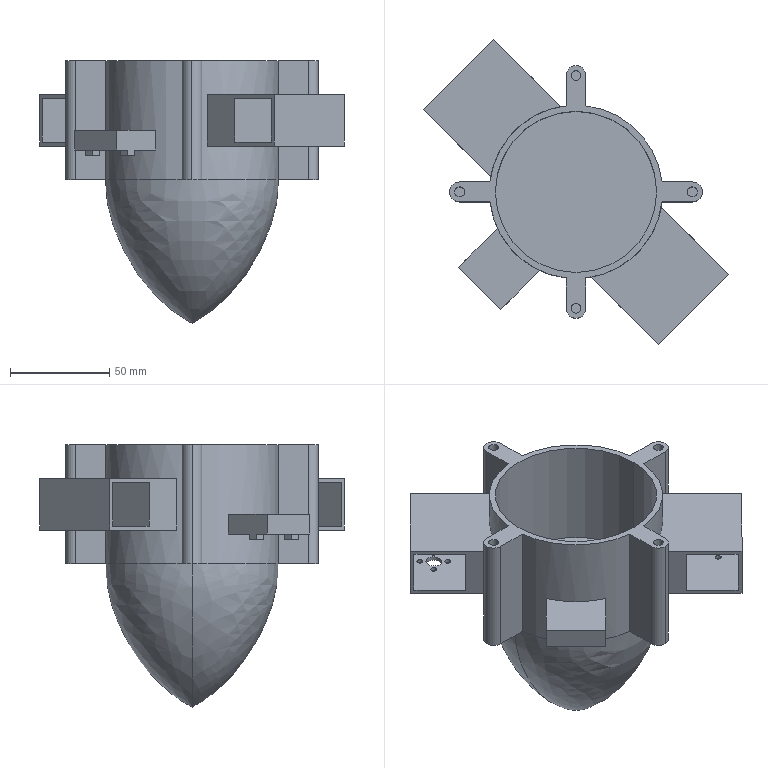Part | SolidWorks | features ICE 10, MirrorPattern 2, CirPattern 1, Extrusion 1, Fillet 1, HoleWzd 1, Revolution 1 | 1 solid | 101 faces | box 153.584 x 153.584 x 132.279 mm | volume 420410 mm3 | plane 49 | cylinder 46 | cone 4 | spline 2 | commonest cylinder face diameters 3 x16 5 x8 10 x8 1.6 x4 8 x4 87.2 x4